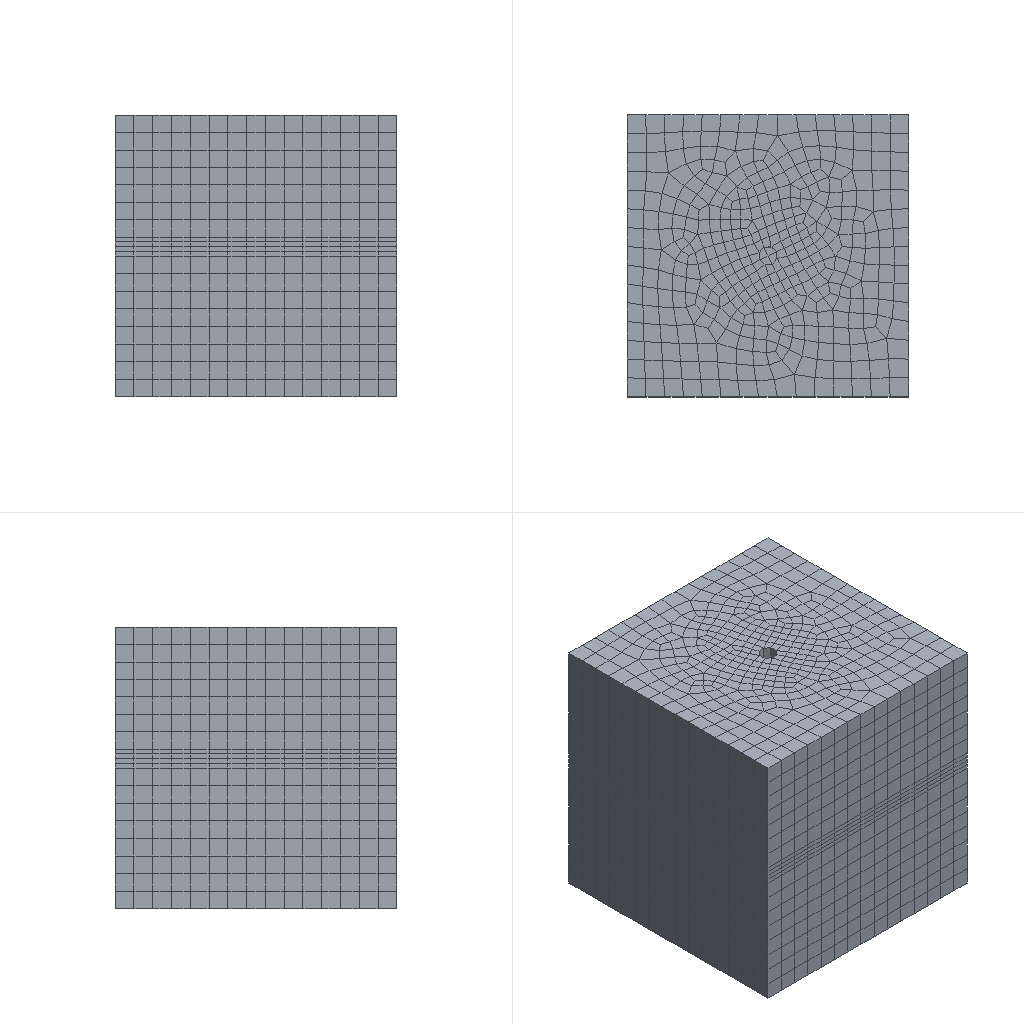Simulation study | abaqus
Set-up summary:
category,name,step,type,value,unit,region
solver,abaqus
solver,version,,,Abaqus/Standard 3DEXPERIENCE R2017x
units,not stated in the deck,,not stated
analysis,deck,,geostatic,geostatic
load_step,Step-geo,Step-geo,geostatic
load_step,Step-1,Step-1,soils
load_step,Step-2,Step-2,soils
load_step,Step-3,Step-3,soils
load_step,requested,,,4
mesh,nodes,,,8869
mesh,elements,,,7803
element_type,C3D8P,,solid,7803
load,load commands in deck,,count,3
bc,support commands in deck,,count,3
material,MATERIAL-1,,in results
check,setup vs results,,match,"per instance, exact: element labels, types and connectivity; labels of the nodes the elements use; coordinates of those nodes at SINGLE_PRECISION in 1 of 1 instance(s)"
Abaqus input file, long lists of numbers shortened:
*Heading
** Job name: Job-3 Model name: Model-1-Copy
** Generated by: Abaqus/CAE 2017
*Preprint, echo=NO, model=NO, history=NO, contact=NO
**
** PARTS
**
*Part, name=Part-1
*Node
      1,          30.,         -30.,          15.
      2,          30.,           0.,          15.
** (8867 more lines like these left out)
*Element, type=C3D8P
   1,  431,  688,  389,  381, 2903, 3160, 2861, 2853
   2,  419,  424,  464,  445, 2891, 2896, 2936, 2917
** (7801 more lines like these left out)
*Nset, nset=Set-1, generate
    1,  8869,     1
*Elset, elset=Set-1, generate
    1,  7803,     1
** Section: Section-1
*Solid Section, elset=Set-1, material=Material-1
,
*End Part
**
**
** ASSEMBLY
**
*Assembly, name=Assembly
**
*Instance, name=Part-1-1, part=Part-1
*End Instance
**
*Nset, nset=Set-1, instance=Part-1-1
    1,    2,    3,    4,    5,   16,   17,   18,   19,   20,   21,   22,   23,   24,   25,   26
   27,   28,   29,   30,   31,   32,   33,   34,   35,   36,   37,   38,   39,   40,   41,   42
** (248 more lines like these left out)
*Elset, elset=Set-1, instance=Part-1-1, generate
 4500,  7803,     1
*Nset, nset=Set-3, instance=Part-1-1
    1,    4,   18,   19,   62,   63,   64,   65,   66,   67,   68,   69,   70,   71,   72,   73
   74,   75,  258,  259,  260,  261,  262,  263,  264,  265,  266,  267,  268,  269,  270,  271
** (7 more lines like these left out)
*Elset, elset=Set-3, instance=Part-1-1
 4512, 4548, 4558, 4747, 4770, 4781, 4791, 4814, 4815, 4831, 4842, 4847, 4853, 4863, 4887, 4925
 4961, 4971, 5160, 5183, 5194, 5204, 5227, 5228, 5244, 5255, 5260, 5266, 5276, 5300, 5338, 5374
** (6 more lines like these left out)
*Nset, nset=Set-4, instance=Part-1-1
    1,    2,    3,    4,    5,   11,   12,   13,   14,   15,   16,   17,   18,   19,   20,   21
   22,   23,   24,   25,   26,   27,   28,   29,   30,   31,   32,   33,   34,   35,   36,   37
** (249 more lines like these left out)
*Elset, elset=Set-4, instance=Part-1-1, generate
 4500,  7803,     1
*Nset, nset=Set-5, instance=Part-1-1
    1,    2,    3,    4,    5,   11,   12,   13,   14,   15,   16,   17,   18,   19,   20,   21
   22,   23,   24,   25,   26,   27,   28,   29,   30,   31,   32,   33,   34,   35,   36,   37
** (249 more lines like these left out)
*Elset, elset=Set-5, instance=Part-1-1, generate
 4500,  7803,     1
*Nset, nset=Set-6, instance=Part-1-1
    1,    2,    3,    4,   16,   17,   18,   19,   20,   21,   22,   23,   24,   25,   26,   27
   28,   29,   30,   31,   32,   33,   48,   49,   50,   51,   52,   53,   54,   55,   56,   57
** (16 more lines like these left out)
*Elset, elset=Set-6, instance=Part-1-1
 4508, 4531, 4540, 4548, 4555, 4556, 4558, 4731, 4739, 4775, 4802, 4804, 4809, 4812, 4823, 4826
 4830, 4832, 4836, 4840, 4841, 4843, 4845, 4849, 4855, 4856, 4857, 4858, 4862, 4867, 4921, 4944
** (13 more lines like these left out)
*Nset, nset=Set-7, instance=Part-1-1
    1,    2,    3,    4,   16,   17,   18,   19,   34,   35,   36,   37,   38,   39,   40,   41
   42,   43,   44,   45,   46,   47,   62,   63,   64,   65,   66,   67,   68,   69,   70,   71
** (16 more lines like these left out)
*Elset, elset=Set-7, instance=Part-1-1
 4512, 4516, 4531, 4540, 4548, 4558, 4747, 4770, 4776, 4781, 4791, 4794, 4795, 4803, 4814, 4815
 4821, 4831, 4838, 4839, 4842, 4844, 4847, 4851, 4853, 4860, 4861, 4863, 4865, 4887, 4925, 4929
** (13 more lines like these left out)
*Nset, nset=Set-8, instance=Part-1-1
   16,   17,   18,   19,  279,  280,  281,  282,  283,  284,  285,  286,  287,  288,  289,  290
  291,  292,  293,  294,  295,  296,  297,  298,  299,  300,  301,  302,  303,  304,  305,  306
** (26 more lines like these left out)
*Elset, elset=Set-8, instance=Part-1-1, generate
 7391,  7803,     1
*Nset, nset=Set-9, instance=Part-1-1
    1,    2,    3,    4,    5,    6,    7,    8,    9,   10,   11,   12,   13,   14,   15,   16
   17,   18,   19,   20,   21,   22,   23,   24,   25,   26,   27,   28,   29,   30,   31,   32
** (251 more lines like these left out)
*Elset, elset=Set-9, instance=Part-1-1
   28,   37,   45,   55,  437,  446,  454,  464,  846,  855,  863,  873, 1255, 1264, 1272, 1282
 1659, 1664, 1673, 1681, 1691, 2068, 2073, 2082, 2090, 2100, 2477, 2482, 2491, 2499, 2509, 2886
** (208 more lines like these left out)
*Nset, nset=Set-10, instance=Part-1-1
    1,    2,    3,    4,    5,    6,    7,    8,    9,   10,   11,   12,   13,   14,   15,   16
   17,   18,   19,   20,   21,   22,   23,   24,   25,   26,   27,   28,   29,   30,   31,   32
** (251 more lines like these left out)
*Elset, elset=Set-10, instance=Part-1-1
   28,   37,   45,   55,  437,  446,  454,  464,  846,  855,  863,  873, 1255, 1264, 1272, 1282
 1659, 1664, 1673, 1681, 1691, 2068, 2073, 2082, 2090, 2100, 2477, 2482, 2491, 2499, 2509, 2886
** (208 more lines like these left out)
*Nset, nset=Set-11, instance=Part-1-1
    1,    2,    3,    4,   16,   17,   18,   19,   20,   21,   22,   23,   24,   25,   26,   27
   28,   29,   30,   31,   32,   33,   48,   49,   50,   51,   52,   53,   54,   55,   56,   57
** (16 more lines like these left out)
*Elset, elset=Set-11, instance=Part-1-1
 4508, 4531, 4540, 4548, 4555, 4556, 4558, 4731, 4739, 4775, 4802, 4804, 4809, 4812, 4823, 4826
 4830, 4832, 4836, 4840, 4841, 4843, 4845, 4849, 4855, 4856, 4857, 4858, 4862, 4867, 4921, 4944
** (13 more lines like these left out)
*Nset, nset=Set-12, instance=Part-1-1
    1,    2,    3,    4,   16,   17,   18,   19,   34,   35,   36,   37,   38,   39,   40,   41
   42,   43,   44,   45,   46,   47,   62,   63,   64,   65,   66,   67,   68,   69,   70,   71
** (16 more lines like these left out)
*Elset, elset=Set-12, instance=Part-1-1
 4512, 4516, 4531, 4540, 4548, 4558, 4747, 4770, 4776, 4781, 4791, 4794, 4795, 4803, 4814, 4815
 4821, 4831, 4838, 4839, 4842, 4844, 4847, 4851, 4853, 4860, 4861, 4863, 4865, 4887, 4925, 4929
** (13 more lines like these left out)
*Nset, nset=Set-13, instance=Part-1-1
   16,   17,   18,   19,  279,  280,  281,  282,  283,  284,  285,  286,  287,  288,  289,  290
  291,  292,  293,  294,  295,  296,  297,  298,  299,  300,  301,  302,  303,  304,  305,  306
** (26 more lines like these left out)
*Elset, elset=Set-13, instance=Part-1-1, generate
 7391,  7803,     1
*Nset, nset=Set-14, instance=Part-1-1
   16,   17,   18,   19,  279,  280,  281,  282,  283,  284,  285,  286,  287,  288,  289,  290
  291,  292,  293,  294,  295,  296,  297,  298,  299,  300,  301,  302,  303,  304,  305,  306
** (26 more lines like these left out)
*Elset, elset=Set-14, instance=Part-1-1, generate
 7391,  7803,     1
*Nset, nset=Set-15, instance=Part-1-1
    1,    2,    3,    4,    5,   16,   17,   18,   19,   20,   21,   22,   23,   24,   25,   26
   27,   28,   29,   30,   31,   32,   33,   34,   35,   36,   37,   38,   39,   40,   41,   42
** (248 more lines like these left out)
*Elset, elset=Set-15, instance=Part-1-1, generate
 4500,  7803,     1
*Nset, nset=Set-16, instance=Part-1-1
   16,   17,   18,   19,  279,  280,  281,  282,  283,  284,  285,  286,  287,  288,  289,  290
  291,  292,  293,  294,  295,  296,  297,  298,  299,  300,  301,  302,  303,  304,  305,  306
** (26 more lines like these left out)
*Elset, elset=Set-16, instance=Part-1-1, generate
 7391,  7803,     1
*Nset, nset=Set-17, instance=Part-1-1
   16,   17,   18,   19,  279,  280,  281,  282,  283,  284,  285,  286,  287,  288,  289,  290
  291,  292,  293,  294,  295,  296,  297,  298,  299,  300,  301,  302,  303,  304,  305,  306
** (26 more lines like these left out)
*Elset, elset=Set-17, instance=Part-1-1, generate
 7391,  7803,     1
*Nset, nset=Set-18, instance=Part-1-1
   16,   17,   18,   19,  279,  280,  281,  282,  283,  284,  285,  286,  287,  288,  289,  290
  291,  292,  293,  294,  295,  296,  297,  298,  299,  300,  301,  302,  303,  304,  305,  306
** (26 more lines like these left out)
*Elset, elset=Set-18, instance=Part-1-1, generate
 7391,  7803,     1
*Nset, nset=Set-19, instance=Part-1-1
    2,    3,   16,   17,   34,   35,   36,   37,   38,   39,   40,   41,   42,   43,   44,   45
   46,   47,  251,  252,  253,  254,  255,  256,  257,  272,  273,  274,  275,  276,  277,  278
** (7 more lines like these left out)
*Elset, elset=Set-19, instance=Part-1-1
 4516, 4531, 4540, 4776, 4794, 4795, 4803, 4821, 4838, 4839, 4844, 4851, 4860, 4861, 4865, 4929
 4944, 4953, 5189, 5207, 5208, 5216, 5234, 5251, 5252, 5257, 5264, 5273, 5274, 5278, 5342, 5357
** (6 more lines like these left out)
*Nset, nset=Set-20, instance=Part-1-1
    1,    2,   17,   18,   20,   21,   22,   23,   24,   25,   26,   27,   28,   29,   30,   31
   32,   33,  265,  266,  267,  268,  269,  270,  271,  272,  273,  274,  275,  276,  277,  278
** (7 more lines like these left out)
*Elset, elset=Set-20, instance=Part-1-1
 4531, 4555, 4556, 4558, 4731, 4775, 4809, 4826, 4830, 4832, 4836, 4843, 4849, 4856, 4862, 4944
 4968, 4969, 4971, 5144, 5188, 5222, 5239, 5243, 5245, 5249, 5256, 5262, 5269, 5275, 5357, 5381
** (6 more lines like these left out)
*Nset, nset=Set-21, instance=Part-1-1
    1,    2,    3,    4,   16,   17,   18,   19,   20,   21,   22,   23,   24,   25,   26,   27
   28,   29,   30,   31,   32,   33,   48,   49,   50,   51,   52,   53,   54,   55,   56,   57
** (16 more lines like these left out)
*Elset, elset=Set-21, instance=Part-1-1
 4508, 4531, 4540, 4548, 4555, 4556, 4558, 4731, 4739, 4775, 4802, 4804, 4809, 4812, 4823, 4826
 4830, 4832, 4836, 4840, 4841, 4843, 4845, 4849, 4855, 4856, 4857, 4858, 4862, 4867, 4921, 4944
** (13 more lines like these left out)
*Nset, nset=Set-22, instance=Part-1-1, generate
    1,  8869,     1
*Elset, elset=Set-22, instance=Part-1-1, generate
    1,  7803,     1
*Nset, nset=Set-23, instance=Part-1-1, generate
    1,  8869,     1
*Elset, elset=Set-23, instance=Part-1-1, generate
    1,  7803,     1
*Nset, nset=Set-24, instance=Part-1-1, generate
    1,  8869,     1
*Elset, elset=Set-24, instance=Part-1-1, generate
    1,  7803,     1
*Nset, nset=Set-25, instance=Part-1-1
    1,    2,    3,    4,    7,    8,    9,   10,   12,   13,   14,   15,   16,   17,   18,   19
   20,   21,   22,   23,   24,   25,   26,   27,   28,   29,   30,   31,   32,   33,   48,   49
** (38 more lines like these left out)
*Elset, elset=Set-25, instance=Part-1-1
    5,   28,   37,   45,   52,   53,   55,  228,  236,  272,  299,  301,  306,  309,  320,  323
  327,  329,  333,  337,  338,  340,  342,  346,  352,  353,  354,  355,  359,  364,  414,  437
** (34 more lines like these left out)
*Nset, nset=Set-26, instance=Part-1-1
    1,    2,    3,    4,    7,    8,    9,   10,   12,   13,   14,   15,   16,   17,   18,   19
   34,   35,   36,   37,   38,   39,   40,   41,   42,   43,   44,   45,   46,   47,   62,   63
** (38 more lines like these left out)
*Elset, elset=Set-26, instance=Part-1-1
    9,   13,   28,   37,   45,   55,  244,  267,  273,  278,  288,  291,  292,  300,  311,  312
  318,  328,  335,  336,  339,  341,  344,  348,  350,  357,  358,  360,  362,  384,  418,  422
** (34 more lines like these left out)
*Nset, nset=Set-27, instance=Part-1-1
   11,   12,   13,   14,   15,   16,   17,   18,   19,  188,  189,  190,  191,  192,  193,  194
  195,  196,  197,  198,  199,  200,  201,  202,  203,  204,  205,  206,  207,  208,  209,  210
** (54 more lines like these left out)
*Elset, elset=Set-27, instance=Part-1-1
 4091, 4092, 4093, 4094, 4095, 4096, 4097, 4098, 4099, 4100, 4101, 4102, 4103, 4104, 4105, 4106
 4107, 4108, 4109, 4110, 4111, 4112, 4113, 4114, 4115, 4116, 4117, 4118, 4119, 4120, 4121, 4122
** (50 more lines like these left out)
*Nset, nset=Set-28, instance=Part-1-1
   12,   13,   14,   15,   16,   17,   18,   19,  195,  196,  197,  198,  199,  200,  201,  202
  203,  204,  205,  206,  207,  208,  209,  210,  211,  212,  213,  214,  215,  216,  217,  218
** (30 more lines like these left out)
*Elset, elset=Set-28, instance=Part-1-1
 4095, 4099, 4103, 4118, 4127, 4135, 4142, 4143, 4145, 4318, 4326, 4334, 4357, 4362, 4363, 4368
 4378, 4381, 4382, 4389, 4390, 4391, 4396, 4399, 4401, 4402, 4408, 4410, 4413, 4417, 4418, 4419
** (28 more lines like these left out)
*Nset, nset=Set-29, instance=Part-1-1
   11,   12,   13,   14,   15,   16,   17,   18,   19,  188,  189,  190,  191,  192,  193,  194
  195,  196,  197,  198,  199,  200,  201,  202,  203,  204,  205,  206,  207,  208,  209,  210
** (54 more lines like these left out)
*Elset, elset=Set-29, instance=Part-1-1
 4091, 4092, 4093, 4094, 4095, 4096, 4097, 4098, 4099, 4100, 4101, 4102, 4103, 4104, 4105, 4106
 4107, 4108, 4109, 4110, 4111, 4112, 4113, 4114, 4115, 4116, 4117, 4118, 4119, 4120, 4121, 4122
** (50 more lines like these left out)
*Nset, nset=Set-30, instance=Part-1-1
  12,  13,  14,  15,  16,  17,  18,  19, 195, 196, 197, 198, 199, 200, 201, 202
 203, 204, 205, 206, 207, 208, 209, 210, 211, 212, 213, 214, 215, 216, 217, 218
** (6 more lines like these left out)
*Elset, elset=Set-30, instance=Part-1-1
 4095, 4099, 4103, 4118, 4127, 4135, 4142, 4143, 4145, 4318, 4326, 4334, 4357, 4362, 4363, 4368
 4378, 4381, 4382, 4389, 4390, 4391, 4396, 4399, 4401, 4402, 4408, 4410, 4413, 4417, 4418, 4419
** (5 more lines like these left out)
*Nset, nset=Set-31, instance=Part-1-1
    5,   76,   77,   78,   79,   80,   81,   82, 2030
*Elset, elset=Set-31, instance=Part-1-1, generate
 4500,  4503,     1
*Nset, nset=Set-32, instance=Part-1-1
   16,   17,   18,   19,  279,  280,  281,  282,  283,  284,  285,  286,  287,  288,  289,  290
  291,  292,  293,  294,  295,  296,  297,  298,  299,  300,  301,  302,  303,  304,  305,  306
** (26 more lines like these left out)
*Elset, elset=Set-32, instance=Part-1-1, generate
 7391,  7803,     1
*Nset, nset=Set-33, instance=Part-1-1
   11,   12,   13,   14,   15,   16,   17,   18,   19,  188,  189,  190,  191,  192,  193,  194
  195,  196,  197,  198,  199,  200,  201,  202,  203,  204,  205,  206,  207,  208,  209,  210
** (54 more lines like these left out)
*Elset, elset=Set-33, instance=Part-1-1
 4091, 4092, 4093, 4094, 4095, 4096, 4097, 4098, 4099, 4100, 4101, 4102, 4103, 4104, 4105, 4106
 4107, 4108, 4109, 4110, 4111, 4112, 4113, 4114, 4115, 4116, 4117, 4118, 4119, 4120, 4121, 4122
** (50 more lines like these left out)
*Nset, nset=_PickedSet40, internal, instance=Part-1-1, generate
    1,  8869,     1
*Elset, elset=_PickedSet40, internal, instance=Part-1-1, generate
    1,  7803,     1
*Elset, elset=_Surf-3_S1, internal, instance=Part-1-1, generate
 4500,  4503,     1
*Surface, type=ELEMENT, name=Surf-3
_Surf-3_S1, S1
*Elset, elset=_Surf-5_S5, internal, instance=Part-1-1
   16,   20,   31,   39,  425,  429,  440,  448,  834,  838,  849,  857, 1243, 1247, 1258, 1266
*Elset, elset=_Surf-5_S4, internal, instance=Part-1-1
   23,   33,   42,  432,  442,  451,  841,  851,  860, 1250, 1260, 1269
*Elset, elset=_Surf-5_S6, internal, instance=Part-1-1, generate
   44,  1271,   409
*Surface, type=ELEMENT, name=Surf-5
_Surf-5_S5, S5
_Surf-5_S4, S4
_Surf-5_S6, S6
*Elset, elset=_Surf-6_S5, internal, instance=Part-1-1
   16,   20,   31,   39,  425,  429,  440,  448,  834,  838,  849,  857, 1243, 1247, 1258, 1266
*Elset, elset=_Surf-6_S4, internal, instance=Part-1-1
   23,   33,   42,  432,  442,  451,  841,  851,  860, 1250, 1260, 1269
*Elset, elset=_Surf-6_S6, internal, instance=Part-1-1, generate
   44,  1271,   409
*Elset, elset=_Surf-6_S1, internal, instance=Part-1-1, generate
 4500,  4503,     1
*Surface, type=ELEMENT, name=Surf-6
_Surf-6_S5, S5
_Surf-6_S4, S4
_Surf-6_S6, S6
_Surf-6_S1, S1
*Elset, elset=_Surf-7_S5, internal, instance=Part-1-1
   16,   20,   31,   39,  425,  429,  440,  448,  834,  838,  849,  857, 1243, 1247, 1258, 1266
*Elset, elset=_Surf-7_S4, internal, instance=Part-1-1
   23,   33,   42,  432,  442,  451,  841,  851,  860, 1250, 1260, 1269
*Elset, elset=_Surf-7_S6, internal, instance=Part-1-1, generate
   44,  1271,   409
*Surface, type=ELEMENT, name=Surf-7
_Surf-7_S5, S5
_Surf-7_S4, S4
_Surf-7_S6, S6
*Elset, elset=_Surf-8_S5, internal, instance=Part-1-1
   16,   20,   31,   39,  425,  429,  440,  448,  834,  838,  849,  857, 1243, 1247, 1258, 1266
*Elset, elset=_Surf-8_S4, internal, instance=Part-1-1
   23,   33,   42,  432,  442,  451,  841,  851,  860, 1250, 1260, 1269
*Elset, elset=_Surf-8_S6, internal, instance=Part-1-1, generate
   44,  1271,   409
*Elset, elset=_Surf-8_S1, internal, instance=Part-1-1, generate
 4500,  4503,     1
*Surface, type=ELEMENT, name=Surf-8
_Surf-8_S5, S5
_Surf-8_S4, S4
_Surf-8_S6, S6
_Surf-8_S1, S1
*Elset, elset=_Surf-9_S5, internal, instance=Part-1-1
   16,   20,   31,   39,  425,  429,  440,  448,  834,  838,  849,  857, 1243, 1247, 1258, 1266
*Elset, elset=_Surf-9_S4, internal, instance=Part-1-1
   23,   33,   42,  432,  442,  451,  841,  851,  860, 1250, 1260, 1269
*Elset, elset=_Surf-9_S6, internal, instance=Part-1-1, generate
   44,  1271,   409
*Elset, elset=_Surf-9_S1, internal, instance=Part-1-1, generate
 4500,  4503,     1
*Surface, type=ELEMENT, name=Surf-9
_Surf-9_S5, S5
_Surf-9_S4, S4
_Surf-9_S6, S6
_Surf-9_S1, S1
*Enrichment, name=Crack-1, type=PROPAGATION CRACK, elset=_PickedSet40, interaction=IntProp-1
*End Assembly
*Amplitude, name=Amp-1
             0.,              0.,              1.,              1.
**
** MATERIALS
**
*Material, name=Material-1
*Damage Initiation, criterion=MAXPS
2.,
*Damage Evolution, type=DISPLACEMENT
 1e-06,
*Damage Stabilization
1e-05
*Density
 3e-09,
*Elastic
16000., 0.25
*Fluid Leakoff
 1e-05, 1e-05
*Gap Flow
 0.001,
*Permeability, specific=1e-09
 0.0001, 0.2
**
** INTERACTION PROPERTIES
**
*Surface Interaction, name=IntProp-1
1.,
**
** BOUNDARY CONDITIONS
**
** Name: BC-1 Type: 位移/转角
*Boundary
Set-25, 1, 1
** Name: BC-2 Type: 位移/转角
*Boundary
Set-26, 2, 2
** Name: BC-3 Type: 位移/转角
*Boundary
Set-33, 3, 3
**
** PREDEFINED FIELDS
**
** Name: Predefined Field-1   Type: Stress
*Initial Conditions, type=STRESS
Set-22, -12., -16., 0., 0., 0., 0.
** Name: Predefined Field-2   Type: Pore pressure
*Initial Conditions, TYPE=PORE PRESSURE
Set-23, 4.
** Name: Predefined Field-3   Type: Void ratio
*Initial Conditions, TYPE=RATIO
Set-24, 0.3
** ----------------------------------------------------------------
**
** STEP: Step-geo
**
*Step, name=Step-geo, nlgeom=YES, unsymm=YES
*Geostatic
**
** LOADS
**
** Name: Load-2   Type: Gravity
*Dload
, GRAV, 9800., 0., 1., 0.
**
** OUTPUT REQUESTS
**
*Restart, write, frequency=0
**
** FIELD OUTPUT: F-Output-2
**
*Output, field
*Node Output
U, V
*Element Output, directions=YES
MISES, S
*Output, history, frequency=0
*End Step
** ----------------------------------------------------------------
**
** STEP: Step-1
**
*Step, name=Step-1, nlgeom=YES, inc=10000, unsymm=YES
*Soils, consolidation, end=PERIOD, utol=1e+07, creep=none, stabilize=0.0002, allsdtol=0.05, continue=NO
0.001, 1., 1e-05, 1.,
**
** LOADS
**
** Name: Load-1   Type: Surface pore fluid
*Dsflow, amplitude=Amp-1
Surf-8, S, 0.01
**
** CONTROLS
**
*Controls, reset
**
** OUTPUT REQUESTS
**
*Restart, write, frequency=0
**
** FIELD OUTPUT: F-Output-1
**
*Output, field
*Node Output
CF, PHILSM, POR, PSILSM, RF, U
*Element Output, directions=YES
E, LE, MISES, MISESMAX, S, SAT, SDEG, VOIDR
*Contact Output
CSDMG, CSTRESS, PFL, PFLA, PTL, PTLA
**
** FIELD OUTPUT: F-Output-2
**
*Node Output
U, V
*Element Output, directions=YES
MISES, S
**
** HISTORY OUTPUT: H-Output-1
**
*Output, history, variable=PRESELECT
*End Step
** ----------------------------------------------------------------
**
** STEP: Step-2
**
*Step, name=Step-2, nlgeom=YES, inc=1000
*Soils, consolidation, end=PERIOD, utol=100000., creep=none, stabilize=0.0002, allsdtol=0.05, continue=NO
0.001, 1., 1e-05, 1.,
**
** LOADS
**
** Name: Load-1   Type: Surface pore fluid
*Dsflow, op=NEW
**
** OUTPUT REQUESTS
**
*Restart, write, frequency=0
**
** FIELD OUTPUT: F-Output-1
**
*Output, field
*Node Output
CF, PHILSM, POR, PSILSM, RF, U
*Element Output, directions=YES
E, LE, MISES, MISESMAX, S, SAT, SDEG, VOIDR
*Contact Output
CSDMG, CSTRESS, PFL, PFLA, PTL, PTLA
**
** FIELD OUTPUT: F-Output-2
**
*Node Output
U, V
*Element Output, directions=YES
MISES, S
**
** HISTORY OUTPUT: H-Output-1
**
*Output, history, variable=PRESELECT
*End Step
** ----------------------------------------------------------------
**
** STEP: Step-3
**
*Step, name=Step-3, nlgeom=YES, inc=1000
*Soils, consolidation, end=PERIOD, utol=10000., creep=none, stabilize=0.0002, allsdtol=0.05, continue=NO
0.001, 1., 1e-06, 1.,
**
** LOADS
**
** Name: Load-1-Copy   Type: Surface pore fluid
*Dsflow, amplitude=Amp-1
Surf-9, S, 0.005
**
** OUTPUT REQUESTS
**
*Restart, write, frequency=0
**
** FIELD OUTPUT: F-Output-1
**
*Output, field
*Node Output
CF, PHILSM, POR, PSILSM, RF, U
*Element Output, directions=YES
E, LE, MISES, MISESMAX, S, SAT, SDEG, VOIDR
*Contact Output
CSDMG, CSTRESS, PFL, PFLA, PTL, PTLA
**
** FIELD OUTPUT: F-Output-2
**
*Node Output
U, V
*Element Output, directions=YES
MISES, S
**
** HISTORY OUTPUT: H-Output-1
**
*Output, history, variable=PRESELECT
*End Step
Results summary:
result,step,,completed,increments=1 time=1.0/1.0
result,step,,completed,increments=18 time=1.0/1.0
result,step,,completed,increments=12 time=1.0/1.0
result,step,,partial,increments=14 time=0.4723/1.0
result,analysis,,,"soils, consolidation"
result,last_loadstep,,,4
result,primary field,,,"U, POR"
result,reaction total,,FX,-3e-06,model units
result,reaction total,,FY,-0.7926,model units
result,reaction total,,FZ,2.1e-05,model units